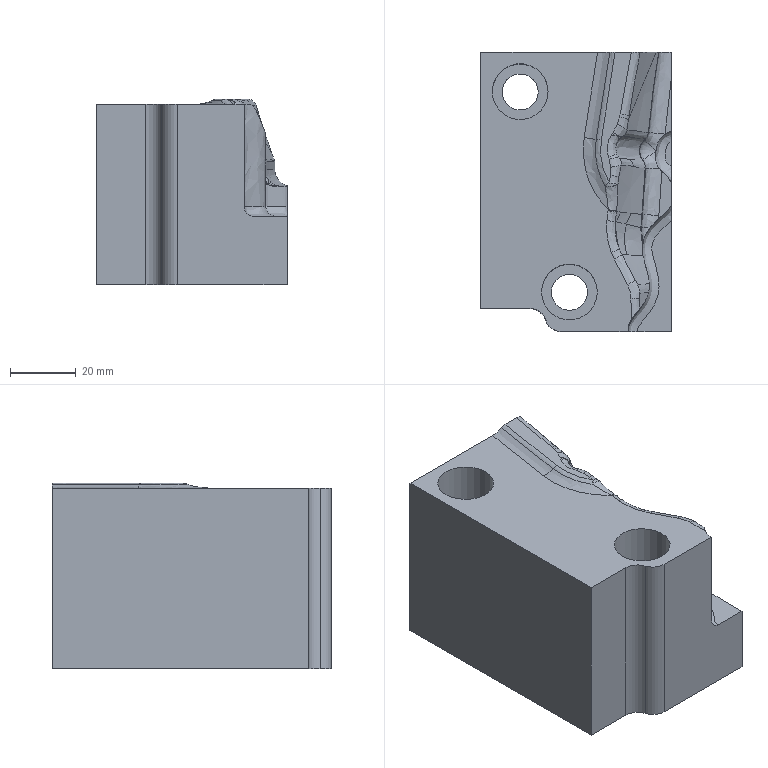Part | STEP file | 1 solid | 89 faces | box 58 x 85 x 56.501 mm | volume 217785 mm3 | spline 71 | plane 12 | cylinder 6 | commonest cylinder face diameters 10 x2 11 x2 17 x2